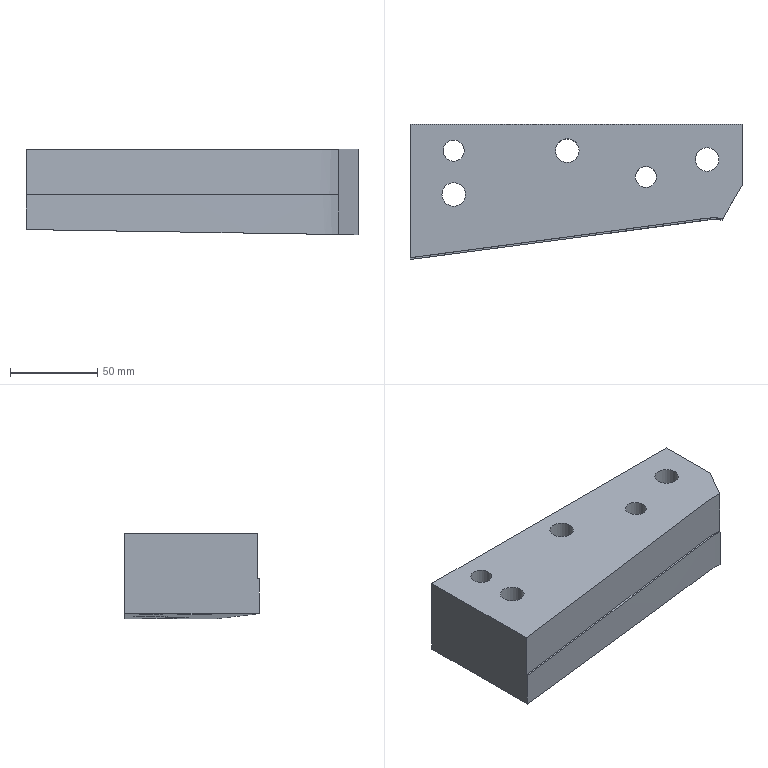Part | NX | features solid 2 | 1 solid | 24 faces | box 190 x 77.202 x 49 mm | volume 533437 mm3 | plane 12 | cylinder 10 | spline 2 | commonest cylinder face diameters 13.5 x3 19.5 x3 12 x2 13 x2
STEP:
#1=CARTESIAN_POINT('',(309.118,134.287,40.));
#2=VERTEX_POINT('',#1);
#3=CARTESIAN_POINT('',(130.,111.807,40.));
#4=VERTEX_POINT('',#3);
#5=CARTESIAN_POINT('',(309.118,134.287,40.));
#6=CARTESIAN_POINT('',(307.251,134.588,40.));
#7=CARTESIAN_POINT('',(303.399,134.795,40.));
#8=CARTESIAN_POINT('',(297.809,134.152,40.));
#9=CARTESIAN_POINT('',(292.221,133.323,40.));
#10=CARTESIAN_POINT('',(284.77,132.284,40.));
#11=CARTESIAN_POINT('',(275.453,130.997,40.));
#12=CARTESIAN_POINT('',(264.266,129.504,40.));
#13=CARTESIAN_POINT('',(253.078,128.021,40.));
#14=CARTESIAN_POINT('',(238.16,126.052,40.));
#15=CARTESIAN_POINT('',(219.511,123.602,40.));
#16=CARTESIAN_POINT('',(197.131,120.668,40.));
#17=CARTESIAN_POINT('',(167.294,116.739,40.));
#18=CARTESIAN_POINT('',(144.918,113.773,40.));
#19=CARTESIAN_POINT('',(130.,111.807,40.));
#20=B_SPLINE_CURVE_WITH_KNOTS('',3,(#5,#6,#7,#8,#9,#10,#11,#12,#13,#14,#15,#16,#17,#18,#19),.UNSPECIFIED.,.F.,.F.,(4,1,1,1,1,1,1,1,1,1,1,1,4),(0.01153,0.01714,0.02276,0.02838,0.034,0.04523,0.05646,0.0677,0.07893,0.1014,0.1239,0.1463,0.1913),.UNSPECIFIED.);
#21=EDGE_CURVE('',#2,#4,#20,.T.);
#22=ORIENTED_EDGE('',*,*,#21,.F.);
#23=CARTESIAN_POINT('',(320.,153.135,40.));
#24=VERTEX_POINT('',#23);
#25=CARTESIAN_POINT('',(85.016,-253.87,40.));
#26=DIRECTION('',(0.5,0.866,0.));
#27=VECTOR('',#26,1000.);
#28=LINE('',#25,#27);
#29=EDGE_CURVE('',#2,#24,#28,.T.);
#30=ORIENTED_EDGE('',*,*,#29,.T.);
#31=CARTESIAN_POINT('',(320.,188.,40.));
#32=VERTEX_POINT('',#31);
#33=CARTESIAN_POINT('',(320.,35.09,40.));
#34=DIRECTION('',(0.,1.,0.));
#35=VECTOR('',#34,1000.);
#36=LINE('',#33,#35);
#37=EDGE_CURVE('',#24,#32,#36,.T.);
#38=ORIENTED_EDGE('',*,*,#37,.T.);
#39=CARTESIAN_POINT('',(130.,188.,40.));
#40=VERTEX_POINT('',#39);
#41=CARTESIAN_POINT('',(-415.478,188.,40.));
#42=DIRECTION('',(1.,0.,0.));
#43=VECTOR('',#42,1000.);
#44=LINE('',#41,#43);
#45=EDGE_CURVE('',#40,#32,#44,.T.);
#46=ORIENTED_EDGE('',*,*,#45,.F.);
#47=CARTESIAN_POINT('',(130.,35.09,40.));
#48=DIRECTION('',(0.,1.,0.));
#49=VECTOR('',#48,1000.);
#50=LINE('',#47,#49);
#51=EDGE_CURVE('',#4,#40,#50,.T.);
#52=ORIENTED_EDGE('',*,*,#51,.F.);
#53=EDGE_LOOP('',(#22,#30,#38,#46,#52));
#54=FACE_BOUND('',#53,.T.);
#55=CARTESIAN_POINT('',(271.,158.,40.));
#56=VERTEX_POINT('',#55);
#57=CARTESIAN_POINT('',(265.,158.,40.));
#58=DIRECTION('',(0.,0.,1.));
#59=DIRECTION('',(1.,0.,0.));
#60=AXIS2_PLACEMENT_3D('',#57,#58,#59);
#61=CIRCLE('',#60,6.);
#62=EDGE_CURVE('',#56,#56,#61,.T.);
#63=ORIENTED_EDGE('',*,*,#62,.F.);
#64=EDGE_LOOP('',(#63));
#65=FACE_BOUND('',#64,.T.);
#66=CARTESIAN_POINT('',(161.,173.,40.));
#67=VERTEX_POINT('',#66);
#68=CARTESIAN_POINT('',(155.,173.,40.));
#69=DIRECTION('',(0.,0.,1.));
#70=DIRECTION('',(1.,0.,0.));
#71=AXIS2_PLACEMENT_3D('',#68,#69,#70);
#72=CIRCLE('',#71,6.);
#73=EDGE_CURVE('',#67,#67,#72,.T.);
#74=ORIENTED_EDGE('',*,*,#73,.F.);
#75=EDGE_LOOP('',(#74));
#76=FACE_BOUND('',#75,.T.);
#77=CARTESIAN_POINT('',(226.75,173.,40.));
#78=VERTEX_POINT('',#77);
#79=CARTESIAN_POINT('',(220.,173.,40.));
#80=DIRECTION('',(0.,0.,1.));
#81=DIRECTION('',(1.,0.,0.));
#82=AXIS2_PLACEMENT_3D('',#79,#80,#81);
#83=CIRCLE('',#82,6.75);
#84=EDGE_CURVE('',#78,#78,#83,.T.);
#85=ORIENTED_EDGE('',*,*,#84,.F.);
#86=EDGE_LOOP('',(#85));
#87=FACE_BOUND('',#86,.T.);
#88=CARTESIAN_POINT('',(161.75,148.,40.));
#89=VERTEX_POINT('',#88);
#90=CARTESIAN_POINT('',(155.,148.,40.));
#91=DIRECTION('',(0.,0.,1.));
#92=DIRECTION('',(1.,0.,0.));
#93=AXIS2_PLACEMENT_3D('',#90,#91,#92);
#94=CIRCLE('',#93,6.75);
#95=EDGE_CURVE('',#89,#89,#94,.T.);
#96=ORIENTED_EDGE('',*,*,#95,.F.);
#97=EDGE_LOOP('',(#96));
#98=FACE_BOUND('',#97,.T.);
#99=CARTESIAN_POINT('',(306.75,168.,40.));
#100=VERTEX_POINT('',#99);
#101=CARTESIAN_POINT('',(300.,168.,40.));
#102=DIRECTION('',(0.,0.,1.));
#103=DIRECTION('',(1.,0.,0.));
#104=AXIS2_PLACEMENT_3D('',#101,#102,#103);
#105=CIRCLE('',#104,6.75);
#106=EDGE_CURVE('',#100,#100,#105,.T.);
#107=ORIENTED_EDGE('',*,*,#106,.F.);
#108=EDGE_LOOP('',(#107));
#109=FACE_BOUND('',#108,.T.);
#110=CARTESIAN_POINT('',(-415.478,35.09,40.));
#111=DIRECTION('',(0.,0.,1.));
#112=DIRECTION('',(1.,0.,0.));
#113=AXIS2_PLACEMENT_3D('',#110,#111,#112);
#114=PLANE('',#113);
#115=ADVANCED_FACE('',(#54,#65,#76,#87,#98,#109),#114,.T.);
#116=CARTESIAN_POINT('',(320.,153.135,-9.));
#117=VERTEX_POINT('',#116);
#118=CARTESIAN_POINT('',(320.,153.135,23.));
#119=DIRECTION('',(0.,0.,1.));
#120=VECTOR('',#119,1000.);
#121=LINE('',#118,#120);
#122=EDGE_CURVE('',#117,#24,#121,.T.);
#123=ORIENTED_EDGE('',*,*,#122,.F.);
#124=CARTESIAN_POINT('',(320.,188.,-9.));
#125=VERTEX_POINT('',#124);
#126=CARTESIAN_POINT('',(320.,-222.,-9.));
#127=DIRECTION('',(0.,-1.,0.));
#128=VECTOR('',#127,1000.);
#129=LINE('',#126,#128);
#130=EDGE_CURVE('',#125,#117,#129,.T.);
#131=ORIENTED_EDGE('',*,*,#130,.F.);
#132=CARTESIAN_POINT('',(320.,188.,-206.));
#133=DIRECTION('',(0.,0.,1.));
#134=VECTOR('',#133,1000.);
#135=LINE('',#132,#134);
#136=EDGE_CURVE('',#125,#32,#135,.T.);
#137=ORIENTED_EDGE('',*,*,#136,.T.);
#138=ORIENTED_EDGE('',*,*,#37,.F.);
#139=EDGE_LOOP('',(#123,#131,#137,#138));
#140=FACE_BOUND('',#139,.T.);
#141=CARTESIAN_POINT('',(320.,105.,2.));
#142=DIRECTION('',(1.,0.,0.));
#143=DIRECTION('',(0.,0.,-1.));
#144=AXIS2_PLACEMENT_3D('',#141,#142,#143);
#145=PLANE('',#144);
#146=ADVANCED_FACE('',(#140),#145,.T.);
#147=CARTESIAN_POINT('',(308.582,133.358,14.));
#148=VERTEX_POINT('',#147);
#149=CARTESIAN_POINT('',(309.118,134.287,14.));
#150=VERTEX_POINT('',#149);
#151=CARTESIAN_POINT('',(326.746,164.819,14.));
#152=DIRECTION('',(0.5,0.866,0.));
#153=VECTOR('',#152,1000.);
#154=LINE('',#151,#153);
#155=EDGE_CURVE('',#148,#150,#154,.T.);
#156=ORIENTED_EDGE('',*,*,#155,.F.);
#157=CARTESIAN_POINT('',(308.582,133.358,-8.82));
#158=VERTEX_POINT('',#157);
#159=CARTESIAN_POINT('',(308.582,133.358,2.57));
#160=DIRECTION('',(0.,0.,-1.));
#161=VECTOR('',#160,1000.);
#162=LINE('',#159,#161);
#163=EDGE_CURVE('',#158,#148,#162,.F.);
#164=ORIENTED_EDGE('',*,*,#163,.F.);
#165=CARTESIAN_POINT('',(-40.023,-470.443,-3.315));
#166=DIRECTION('',(-0.5,-0.866,0.007894));
#167=VECTOR('',#166,1000.);
#168=LINE('',#165,#167);
#169=EDGE_CURVE('',#117,#158,#168,.T.);
#170=ORIENTED_EDGE('',*,*,#169,.F.);
#171=ORIENTED_EDGE('',*,*,#122,.T.);
#172=ORIENTED_EDGE('',*,*,#29,.F.);
#173=CARTESIAN_POINT('',(309.118,134.287,57.));
#174=DIRECTION('',(0.,0.,1.));
#175=VECTOR('',#174,1000.);
#176=LINE('',#173,#175);
#177=EDGE_CURVE('',#150,#2,#176,.T.);
#178=ORIENTED_EDGE('',*,*,#177,.F.);
#179=EDGE_LOOP('',(#156,#164,#170,#171,#172,#178));
#180=FACE_BOUND('',#179,.T.);
#181=CARTESIAN_POINT('',(326.746,164.819,23.));
#182=DIRECTION('',(0.866,-0.5,0.));
#183=DIRECTION('',(0.5,0.866,0.));
#184=AXIS2_PLACEMENT_3D('',#181,#182,#183);
#185=PLANE('',#184);
#186=ADVANCED_FACE('',(#180),#185,.T.);
#187=ORIENTED_EDGE('',*,*,#136,.F.);
#188=CARTESIAN_POINT('',(130.,188.,-6.));
#189=VERTEX_POINT('',#188);
#190=CARTESIAN_POINT('',(-470.225,188.,3.477));
#191=DIRECTION('',(0.9999,0.,-0.01579));
#192=VECTOR('',#191,1000.);
#193=LINE('',#190,#192);
#194=EDGE_CURVE('',#189,#125,#193,.T.);
#195=ORIENTED_EDGE('',*,*,#194,.F.);
#196=CARTESIAN_POINT('',(130.,188.,-206.));
#197=DIRECTION('',(0.,0.,1.));
#198=VECTOR('',#197,1000.);
#199=LINE('',#196,#198);
#200=EDGE_CURVE('',#189,#40,#199,.T.);
#201=ORIENTED_EDGE('',*,*,#200,.T.);
#202=ORIENTED_EDGE('',*,*,#45,.T.);
#203=EDGE_LOOP('',(#187,#195,#201,#202));
#204=FACE_BOUND('',#203,.T.);
#205=CARTESIAN_POINT('',(-470.374,188.,-206.));
#206=DIRECTION('',(0.,-1.,0.));
#207=DIRECTION('',(1.,0.,0.));
#208=AXIS2_PLACEMENT_3D('',#205,#206,#207);
#209=PLANE('',#208);
#210=ADVANCED_FACE('',(#204),#209,.F.);
#211=CARTESIAN_POINT('',(130.,110.798,14.));
#212=VERTEX_POINT('',#211);
#213=CARTESIAN_POINT('',(-190.231,-121.49,14.));
#214=CARTESIAN_POINT('',(-188.654,-121.152,14.));
#215=CARTESIAN_POINT('',(-185.47,-120.627,14.));
#216=CARTESIAN_POINT('',(-180.656,-120.141,14.));
#217=CARTESIAN_POINT('',(-175.882,-119.326,14.));
#218=CARTESIAN_POINT('',(-169.679,-117.528,14.));
#219=CARTESIAN_POINT('',(-162.185,-114.539,14.));
#220=CARTESIAN_POINT('',(-153.086,-111.254,14.));
#221=CARTESIAN_POINT('',(-144.031,-107.845,14.));
#222=CARTESIAN_POINT('',(-136.465,-105.061,14.));
#223=CARTESIAN_POINT('',(-130.418,-102.814,14.));
#224=CARTESIAN_POINT('',(-125.812,-101.329,14.));
#225=CARTESIAN_POINT('',(-121.306,-99.566,14.));
#226=CARTESIAN_POINT('',(-116.876,-97.626,14.));
#227=CARTESIAN_POINT('',(-112.335,-95.923,14.));
#228=CARTESIAN_POINT('',(-107.564,-95.05,14.));
#229=CARTESIAN_POINT('',(-102.756,-94.525,14.));
#230=CARTESIAN_POINT('',(-96.349,-93.771,14.));
#231=CARTESIAN_POINT('',(-89.902,-93.468,14.));
#232=CARTESIAN_POINT('',(-83.452,-93.448,14.));
#233=CARTESIAN_POINT('',(-77.002,-93.469,14.));
#234=CARTESIAN_POINT('',(-68.939,-93.411,14.));
#235=CARTESIAN_POINT('',(-56.04,-93.3,14.));
#236=CARTESIAN_POINT('',(-33.465,-93.184,14.));
#237=CARTESIAN_POINT('',(-7.666,-93.074,14.));
#238=CARTESIAN_POINT('',(14.907,-92.653,14.));
#239=CARTESIAN_POINT('',(27.794,-92.068,14.));
#240=CARTESIAN_POINT('',(40.668,-91.245,14.));
#241=CARTESIAN_POINT('',(51.917,-90.291,14.));
#242=CARTESIAN_POINT('',(61.528,-89.174,14.));
#243=CARTESIAN_POINT('',(67.939,-88.466,14.));
#244=CARTESIAN_POINT('',(79.125,-86.95,14.));
#245=CARTESIAN_POINT('',(95.161,-85.253,14.));
#246=CARTESIAN_POINT('',(114.404,-83.21,14.));
#247=CARTESIAN_POINT('',(133.568,-80.524,14.));
#248=CARTESIAN_POINT('',(152.734,-77.861,14.));
#249=CARTESIAN_POINT('',(171.916,-75.326,14.));
#250=CARTESIAN_POINT('',(191.055,-72.413,14.));
#251=CARTESIAN_POINT('',(207.17,-71.468,14.));
#252=CARTESIAN_POINT('',(219.951,-69.697,14.));
#253=CARTESIAN_POINT('',(232.724,-67.899,14.));
#254=CARTESIAN_POINT('',(248.708,-65.766,14.));
#255=CARTESIAN_POINT('',(267.87,-63.074,14.));
#256=CARTESIAN_POINT('',(287.038,-60.44,14.));
#257=CARTESIAN_POINT('',(301.448,-58.682,14.));
#258=CARTESIAN_POINT('',(310.976,-56.987,14.));
#259=CARTESIAN_POINT('',(314.916,-56.135,14.));
#260=CARTESIAN_POINT('',(318.052,-55.382,14.));
#261=CARTESIAN_POINT('',(320.39,-54.76,14.));
#262=CARTESIAN_POINT('',(322.686,-53.981,14.));
#263=CARTESIAN_POINT('',(325.595,-52.578,14.));
#264=CARTESIAN_POINT('',(328.769,-50.098,14.));
#265=CARTESIAN_POINT('',(332.247,-46.69,14.));
#266=CARTESIAN_POINT('',(335.795,-43.406,14.));
#267=CARTESIAN_POINT('',(343.661,-37.758,14.));
#268=CARTESIAN_POINT('',(355.164,-28.914,14.));
#269=CARTESIAN_POINT('',(370.422,-17.018,14.));
#270=CARTESIAN_POINT('',(383.264,-7.249,14.));
#271=CARTESIAN_POINT('',(392.416,-0.6713,14.));
#272=CARTESIAN_POINT('',(396.953,2.733,14.));
#273=CARTESIAN_POINT('',(398.886,5.372,14.));
#274=CARTESIAN_POINT('',(399.725,7.654,14.));
#275=CARTESIAN_POINT('',(399.76,10.078,14.));
#276=CARTESIAN_POINT('',(399.483,13.317,14.));
#277=CARTESIAN_POINT('',(399.712,17.34,14.));
#278=CARTESIAN_POINT('',(399.612,22.179,14.));
#279=CARTESIAN_POINT('',(399.633,31.854,14.));
#280=CARTESIAN_POINT('',(399.593,46.366,14.));
#281=CARTESIAN_POINT('',(399.637,62.491,14.));
#282=CARTESIAN_POINT('',(399.588,73.779,14.));
#283=CARTESIAN_POINT('',(399.652,79.422,14.));
#284=CARTESIAN_POINT('',(399.59,82.647,14.));
#285=CARTESIAN_POINT('',(399.564,85.065,14.));
#286=CARTESIAN_POINT('',(399.725,87.486,14.));
#287=CARTESIAN_POINT('',(399.756,89.902,14.));
#288=CARTESIAN_POINT('',(399.247,92.301,14.));
#289=CARTESIAN_POINT('',(397.362,95.008,14.));
#290=CARTESIAN_POINT('',(393.635,96.774,14.));
#291=CARTESIAN_POINT('',(389.279,98.826,14.));
#292=CARTESIAN_POINT('',(384.732,100.498,14.));
#293=CARTESIAN_POINT('',(378.765,102.95,14.));
#294=CARTESIAN_POINT('',(362.589,110.229,14.));
#295=CARTESIAN_POINT('',(344.928,118.135,14.));
#296=CARTESIAN_POINT('',(327.281,126.072,14.));
#297=CARTESIAN_POINT('',(319.932,129.381,14.));
#298=CARTESIAN_POINT('',(314.075,132.102,14.));
#299=CARTESIAN_POINT('',(309.387,133.376,14.));
#300=CARTESIAN_POINT('',(304.547,133.785,14.));
#301=CARTESIAN_POINT('',(299.716,133.401,14.));
#302=CARTESIAN_POINT('',(294.929,132.704,14.));
#303=CARTESIAN_POINT('',(288.543,131.8,14.));
#304=CARTESIAN_POINT('',(277.364,130.241,14.));
#305=CARTESIAN_POINT('',(242.2,125.552,14.));
#306=CARTESIAN_POINT('',(184.637,118.048,14.));
#307=CARTESIAN_POINT('',(120.701,109.541,14.));
#308=CARTESIAN_POINT('',(69.531,102.902,14.));
#309=CARTESIAN_POINT('',(40.777,98.94,14.));
#310=CARTESIAN_POINT('',(21.566,96.615,14.));
#311=CARTESIAN_POINT('',(8.743,95.212,14.));
#312=CARTESIAN_POINT('',(-7.301,93.575,14.));
#313=CARTESIAN_POINT('',(-26.625,92.505,14.));
#314=CARTESIAN_POINT('',(-45.971,92.017,14.));
#315=CARTESIAN_POINT('',(-62.09,91.675,14.));
#316=CARTESIAN_POINT('',(-74.987,91.256,14.));
#317=CARTESIAN_POINT('',(-84.664,91.165,14.));
#318=CARTESIAN_POINT('',(-94.319,91.781,14.));
#319=CARTESIAN_POINT('',(-103.929,92.966,14.));
#320=CARTESIAN_POINT('',(-113.495,94.403,14.));
#321=CARTESIAN_POINT('',(-119.856,95.492,14.));
#322=CARTESIAN_POINT('',(-122.997,96.222,14.));
#323=B_SPLINE_CURVE_WITH_KNOTS('',3,(#213,#214,#215,#216,#217,#218,#219,#220,#221,#222,#223,#224,#225,#226,#227,#228,#229,#230,#231,#232,#233,#234,#235,#236,#237,#238,#239,#240,#241,#242,#243,#244,#245,#246,#247,#248,#249,#250,#251,#252,#253,#254,#255,#256,#257,#258,#259,#260,#261,#262,#263,#264,#265,#266,#267,#268,#269,#270,#271,#272,#273,#274,#275,#276,#277,#278,#279,#280,#281,#282,#283,#284,#285,#286,#287,#288,#289,#290,#291,#292,#293,#294,#295,#296,#297,#298,#299,#300,#301,#302,#303,#304,#305,#306,#307,#308,#309,#310,#311,#312,#313,#314,#315,#316,#317,#318,#319,#320,#321,#322),.UNSPECIFIED.,.F.,.F.,(4,1,1,1,1,1,1,1,1,1,1,1,1,1,1,1,1,1,1,1,1,1,1,1,1,1,1,1,1,1,1,1,1,1,1,1,1,1,1,1,1,1,1,1,1,1,1,1,1,1,1,1,1,1,1,1,1,1,1,1,1,1,1,1,1,1,1,1,1,1,1,1,1,1,1,1,1,1,1,1,1,1,1,1,1,1,1,1,1,1,1,1,1,1,1,1,1,1,1,1,1,1,1,1,1,1,1,4),(0.4704,0.4724,0.4745,0.4766,0.4786,0.4828,0.4869,0.491,0.4952,0.4972,0.4993,0.5014,0.5035,0.5055,0.5076,0.5097,0.5117,0.5159,0.5179,0.52,0.5241,0.5283,0.5366,0.5531,0.5614,0.5655,0.5697,0.5779,0.58,0.5821,0.5862,0.5945,0.6028,0.611,0.6193,0.6276,0.6359,0.6441,0.6483,0.6524,0.6607,0.669,0.6772,0.6855,0.6876,0.6897,0.6907,0.6917,0.6928,0.6938,0.6959,0.6979,0.7,0.7021,0.7103,0.7186,0.7269,0.731,0.7331,0.7341,0.7352,0.7362,0.7372,0.7393,0.7414,0.7435,0.7517,0.76,0.7641,0.7662,0.7672,0.7683,0.7693,0.7703,0.7714,0.7724,0.7745,0.7766,0.7786,0.7807,0.7848,0.8014,0.8055,0.8097,0.8117,0.8138,0.8159,0.8179,0.82,0.8221,0.8262,0.8345,0.8676,0.9007,0.9172,0.9338,0.9379,0.9421,0.9503,0.9586,0.9669,0.9752,0.9793,0.9834,0.9876,0.9917,0.9959,1.),.UNSPECIFIED.);
#324=EDGE_CURVE('',#212,#148,#323,.F.);
#325=ORIENTED_EDGE('',*,*,#324,.F.);
#326=CARTESIAN_POINT('',(130.,110.798,-6.));
#327=VERTEX_POINT('',#326);
#328=CARTESIAN_POINT('',(130.,110.798,4.));
#329=DIRECTION('',(0.,0.,-1.));
#330=VECTOR('',#329,1000.);
#331=LINE('',#328,#330);
#332=EDGE_CURVE('',#327,#212,#331,.F.);
#333=ORIENTED_EDGE('',*,*,#332,.F.);
#334=CARTESIAN_POINT('',(130.,110.798,-6.));
#335=CARTESIAN_POINT('',(144.872,112.758,-6.235));
#336=CARTESIAN_POINT('',(167.177,115.715,-6.587));
#337=CARTESIAN_POINT('',(196.921,119.631,-7.057));
#338=CARTESIAN_POINT('',(219.23,122.557,-7.409));
#339=CARTESIAN_POINT('',(237.821,124.999,-7.702));
#340=CARTESIAN_POINT('',(252.692,126.962,-7.937));
#341=CARTESIAN_POINT('',(263.845,128.438,-8.113));
#342=CARTESIAN_POINT('',(274.996,129.934,-8.289));
#343=CARTESIAN_POINT('',(286.146,131.436,-8.465));
#344=CARTESIAN_POINT('',(297.272,133.122,-8.641));
#345=CARTESIAN_POINT('',(304.731,133.922,-8.759));
#346=CARTESIAN_POINT('',(308.582,133.358,-8.82));
#347=B_SPLINE_CURVE_WITH_KNOTS('',3,(#334,#335,#336,#337,#338,#339,#340,#341,#342,#343,#344,#345,#346),.UNSPECIFIED.,.F.,.F.,(4,1,1,1,1,1,1,1,1,1,4),(0.,0.04501,0.06751,0.09001,0.1125,0.1238,0.135,0.1463,0.1575,0.1688,0.18),.UNSPECIFIED.);
#348=EDGE_CURVE('',#327,#158,#347,.T.);
#349=ORIENTED_EDGE('',*,*,#348,.T.);
#350=ORIENTED_EDGE('',*,*,#163,.T.);
#351=EDGE_LOOP('',(#325,#333,#349,#350));
#352=FACE_BOUND('',#351,.T.);
#353=CARTESIAN_POINT('',(308.582,133.358,14.));
#354=CARTESIAN_POINT('',(308.582,133.358,-8.957));
#355=CARTESIAN_POINT('',(306.726,133.63,14.));
#356=CARTESIAN_POINT('',(306.726,133.63,-8.957));
#357=CARTESIAN_POINT('',(302.961,133.768,14.));
#358=CARTESIAN_POINT('',(302.961,133.768,-8.957));
#359=CARTESIAN_POINT('',(297.366,133.074,14.));
#360=CARTESIAN_POINT('',(297.366,133.074,-8.957));
#361=CARTESIAN_POINT('',(291.8,132.254,14.));
#362=CARTESIAN_POINT('',(291.8,132.254,-8.957));
#363=CARTESIAN_POINT('',(284.367,131.218,14.));
#364=CARTESIAN_POINT('',(284.367,131.218,-8.957));
#365=CARTESIAN_POINT('',(275.075,129.937,14.));
#366=CARTESIAN_POINT('',(275.075,129.937,-8.957));
#367=CARTESIAN_POINT('',(263.917,128.449,14.));
#368=CARTESIAN_POINT('',(263.917,128.449,-8.957));
#369=CARTESIAN_POINT('',(252.759,126.97,14.));
#370=CARTESIAN_POINT('',(252.759,126.97,-8.957));
#371=CARTESIAN_POINT('',(237.879,125.006,14.));
#372=CARTESIAN_POINT('',(237.879,125.006,-8.957));
#373=CARTESIAN_POINT('',(219.279,122.563,14.));
#374=CARTESIAN_POINT('',(219.279,122.563,-8.957));
#375=CARTESIAN_POINT('',(196.957,119.636,14.));
#376=CARTESIAN_POINT('',(196.957,119.636,-8.957));
#377=CARTESIAN_POINT('',(167.197,115.718,14.));
#378=CARTESIAN_POINT('',(167.197,115.718,-8.957));
#379=CARTESIAN_POINT('',(144.88,112.759,14.));
#380=CARTESIAN_POINT('',(144.88,112.759,-8.957));
#381=CARTESIAN_POINT('',(130.,110.798,14.));
#382=CARTESIAN_POINT('',(130.,110.798,-8.957));
#383=B_SPLINE_SURFACE_WITH_KNOTS('',3,1,((#353,#354),(#355,#356),(#357,#358),(#359,#360),(#361,#362),(#363,#364),(#365,#366),(#367,#368),(#369,#370),(#371,#372),(#373,#374),(#375,#376),(#377,#378),(#379,#380),(#381,#382)),.SURF_OF_LINEAR_EXTRUSION.,.F.,.F.,.F.,(4,1,1,1,1,1,1,1,1,1,1,1,4),(2,2),(0.8141,0.8165,0.8189,0.8214,0.8238,0.8286,0.8334,0.8382,0.843,0.8526,0.8623,0.8719,0.8912),(0.,1.),.UNSPECIFIED.);
#384=ADVANCED_FACE('',(#352),#383,.T.);
#385=ORIENTED_EDGE('',*,*,#332,.T.);
#386=CARTESIAN_POINT('',(130.,111.807,14.));
#387=VERTEX_POINT('',#386);
#388=CARTESIAN_POINT('',(130.,154.403,14.));
#389=DIRECTION('',(0.,1.,0.));
#390=VECTOR('',#389,1000.);
#391=LINE('',#388,#390);
#392=EDGE_CURVE('',#212,#387,#391,.T.);
#393=ORIENTED_EDGE('',*,*,#392,.T.);
#394=CARTESIAN_POINT('',(130.,111.807,57.));
#395=DIRECTION('',(0.,0.,1.));
#396=VECTOR('',#395,1000.);
#397=LINE('',#394,#396);
#398=EDGE_CURVE('',#387,#4,#397,.T.);
#399=ORIENTED_EDGE('',*,*,#398,.T.);
#400=ORIENTED_EDGE('',*,*,#51,.T.);
#401=ORIENTED_EDGE('',*,*,#200,.F.);
#402=CARTESIAN_POINT('',(130.,-222.,-6.));
#403=DIRECTION('',(0.,-1.,0.));
#404=VECTOR('',#403,1000.);
#405=LINE('',#402,#404);
#406=EDGE_CURVE('',#189,#327,#405,.T.);
#407=ORIENTED_EDGE('',*,*,#406,.T.);
#408=EDGE_LOOP('',(#385,#393,#399,#400,#401,#407));
#409=FACE_BOUND('',#408,.T.);
#410=CARTESIAN_POINT('',(130.,154.403,21.5));
#411=DIRECTION('',(1.,0.,0.));
#412=DIRECTION('',(0.,0.,-1.));
#413=AXIS2_PLACEMENT_3D('',#410,#411,#412);
#414=PLANE('',#413);
#415=ADVANCED_FACE('',(#409),#414,.F.);
#416=ORIENTED_EDGE('',*,*,#106,.T.);
#417=EDGE_LOOP('',(#416));
#418=FACE_BOUND('',#417,.T.);
#419=CARTESIAN_POINT('',(306.75,168.,9.));
#420=VERTEX_POINT('',#419);
#421=CARTESIAN_POINT('',(300.,168.,9.));
#422=DIRECTION('',(0.,0.,1.));
#423=DIRECTION('',(1.,0.,0.));
#424=AXIS2_PLACEMENT_3D('',#421,#422,#423);
#425=CIRCLE('',#424,6.75);
#426=EDGE_CURVE('',#420,#420,#425,.T.);
#427=ORIENTED_EDGE('',*,*,#426,.F.);
#428=EDGE_LOOP('',(#427));
#429=FACE_BOUND('',#428,.T.);
#430=CARTESIAN_POINT('',(300.,168.,94.));
#431=DIRECTION('',(0.,0.,1.));
#432=DIRECTION('',(1.,0.,0.));
#433=AXIS2_PLACEMENT_3D('',#430,#431,#432);
#434=CYLINDRICAL_SURFACE('',#433,6.75);
#435=ADVANCED_FACE('',(#418,#429),#434,.F.);
#436=ORIENTED_EDGE('',*,*,#426,.T.);
#437=EDGE_LOOP('',(#436));
#438=FACE_BOUND('',#437,.T.);
#439=CARTESIAN_POINT('',(309.75,168.,9.));
#440=VERTEX_POINT('',#439);
#441=CARTESIAN_POINT('',(300.,168.,9.));
#442=DIRECTION('',(0.,0.,1.));
#443=DIRECTION('',(1.,0.,0.));
#444=AXIS2_PLACEMENT_3D('',#441,#442,#443);
#445=CIRCLE('',#444,9.75);
#446=EDGE_CURVE('',#440,#440,#445,.T.);
#447=ORIENTED_EDGE('',*,*,#446,.F.);
#448=EDGE_LOOP('',(#447));
#449=FACE_BOUND('',#448,.T.);
#450=CARTESIAN_POINT('',(300.,168.,9.));
#451=DIRECTION('',(0.,0.,1.));
#452=DIRECTION('',(1.,0.,0.));
#453=AXIS2_PLACEMENT_3D('',#450,#451,#452);
#454=PLANE('',#453);
#455=ADVANCED_FACE('',(#438,#449),#454,.F.);
#456=ORIENTED_EDGE('',*,*,#446,.T.);
#457=EDGE_LOOP('',(#456));
#458=FACE_BOUND('',#457,.T.);
#459=CARTESIAN_POINT('',(309.75,168.,-8.838));
#460=VERTEX_POINT('',#459);
#461=CARTESIAN_POINT('',(300.,168.,-8.684));
#462=DIRECTION('',(0.01579,0.,0.9999));
#463=DIRECTION('',(0.9999,0.,-0.01579));
#464=AXIS2_PLACEMENT_3D('',#461,#462,#463);
#465=ELLIPSE('',#464,9.751,9.75);
#466=EDGE_CURVE('',#460,#460,#465,.T.);
#467=ORIENTED_EDGE('',*,*,#466,.F.);
#468=EDGE_LOOP('',(#467));
#469=FACE_BOUND('',#468,.T.);
#470=CARTESIAN_POINT('',(300.,168.,-6.));
#471=DIRECTION('',(0.,0.,1.));
#472=DIRECTION('',(1.,0.,0.));
#473=AXIS2_PLACEMENT_3D('',#470,#471,#472);
#474=CYLINDRICAL_SURFACE('',#473,9.75);
#475=ADVANCED_FACE('',(#458,#469),#474,.F.);
#476=ORIENTED_EDGE('',*,*,#95,.T.);
#477=EDGE_LOOP('',(#476));
#478=FACE_BOUND('',#477,.T.);
#479=CARTESIAN_POINT('',(161.75,148.,9.));
#480=VERTEX_POINT('',#479);
#481=CARTESIAN_POINT('',(155.,148.,9.));
#482=DIRECTION('',(0.,0.,1.));
#483=DIRECTION('',(1.,0.,0.));
#484=AXIS2_PLACEMENT_3D('',#481,#482,#483);
#485=CIRCLE('',#484,6.75);
#486=EDGE_CURVE('',#480,#480,#485,.T.);
#487=ORIENTED_EDGE('',*,*,#486,.F.);
#488=EDGE_LOOP('',(#487));
#489=FACE_BOUND('',#488,.T.);
#490=CARTESIAN_POINT('',(155.,148.,94.));
#491=DIRECTION('',(0.,0.,1.));
#492=DIRECTION('',(1.,0.,0.));
#493=AXIS2_PLACEMENT_3D('',#490,#491,#492);
#494=CYLINDRICAL_SURFACE('',#493,6.75);
#495=ADVANCED_FACE('',(#478,#489),#494,.F.);
#496=ORIENTED_EDGE('',*,*,#486,.T.);
#497=EDGE_LOOP('',(#496));
#498=FACE_BOUND('',#497,.T.);
#499=CARTESIAN_POINT('',(164.75,148.,9.));
#500=VERTEX_POINT('',#499);
#501=CARTESIAN_POINT('',(155.,148.,9.));
#502=DIRECTION('',(0.,0.,1.));
#503=DIRECTION('',(1.,0.,0.));
#504=AXIS2_PLACEMENT_3D('',#501,#502,#503);
#505=CIRCLE('',#504,9.75);
#506=EDGE_CURVE('',#500,#500,#505,.T.);
#507=ORIENTED_EDGE('',*,*,#506,.F.);
#508=EDGE_LOOP('',(#507));
#509=FACE_BOUND('',#508,.T.);
#510=CARTESIAN_POINT('',(155.,148.,9.));
#511=DIRECTION('',(0.,0.,1.));
#512=DIRECTION('',(1.,0.,0.));
#513=AXIS2_PLACEMENT_3D('',#510,#511,#512);
#514=PLANE('',#513);
#515=ADVANCED_FACE('',(#498,#509),#514,.F.);
#516=ORIENTED_EDGE('',*,*,#506,.T.);
#517=EDGE_LOOP('',(#516));
#518=FACE_BOUND('',#517,.T.);
#519=CARTESIAN_POINT('',(164.75,148.,-6.549));
#520=VERTEX_POINT('',#519);
#521=CARTESIAN_POINT('',(155.,148.,-6.395));
#522=DIRECTION('',(0.01579,0.,0.9999));
#523=DIRECTION('',(0.9999,0.,-0.01579));
#524=AXIS2_PLACEMENT_3D('',#521,#522,#523);
#525=ELLIPSE('',#524,9.751,9.75);
#526=EDGE_CURVE('',#520,#520,#525,.T.);
#527=ORIENTED_EDGE('',*,*,#526,.F.);
#528=EDGE_LOOP('',(#527));
#529=FACE_BOUND('',#528,.T.);
#530=CARTESIAN_POINT('',(155.,148.,-6.));
#531=DIRECTION('',(0.,0.,1.));
#532=DIRECTION('',(1.,0.,0.));
#533=AXIS2_PLACEMENT_3D('',#530,#531,#532);
#534=CYLINDRICAL_SURFACE('',#533,9.75);
#535=ADVANCED_FACE('',(#518,#529),#534,.F.);
#536=ORIENTED_EDGE('',*,*,#84,.T.);
#537=EDGE_LOOP('',(#536));
#538=FACE_BOUND('',#537,.T.);
#539=CARTESIAN_POINT('',(226.75,173.,9.));
#540=VERTEX_POINT('',#539);
#541=CARTESIAN_POINT('',(220.,173.,9.));
#542=DIRECTION('',(0.,0.,1.));
#543=DIRECTION('',(1.,0.,0.));
#544=AXIS2_PLACEMENT_3D('',#541,#542,#543);
#545=CIRCLE('',#544,6.75);
#546=EDGE_CURVE('',#540,#540,#545,.T.);
#547=ORIENTED_EDGE('',*,*,#546,.F.);
#548=EDGE_LOOP('',(#547));
#549=FACE_BOUND('',#548,.T.);
#550=CARTESIAN_POINT('',(220.,173.,94.));
#551=DIRECTION('',(0.,0.,1.));
#552=DIRECTION('',(1.,0.,0.));
#553=AXIS2_PLACEMENT_3D('',#550,#551,#552);
#554=CYLINDRICAL_SURFACE('',#553,6.75);
#555=ADVANCED_FACE('',(#538,#549),#554,.F.);
#556=ORIENTED_EDGE('',*,*,#546,.T.);
#557=EDGE_LOOP('',(#556));
#558=FACE_BOUND('',#557,.T.);
#559=CARTESIAN_POINT('',(229.75,173.,9.));
#560=VERTEX_POINT('',#559);
#561=CARTESIAN_POINT('',(220.,173.,9.));
#562=DIRECTION('',(0.,0.,1.));
#563=DIRECTION('',(1.,0.,0.));
#564=AXIS2_PLACEMENT_3D('',#561,#562,#563);
#565=CIRCLE('',#564,9.75);
#566=EDGE_CURVE('',#560,#560,#565,.T.);
#567=ORIENTED_EDGE('',*,*,#566,.F.);
#568=EDGE_LOOP('',(#567));
#569=FACE_BOUND('',#568,.T.);
#570=CARTESIAN_POINT('',(220.,173.,9.));
#571=DIRECTION('',(0.,0.,1.));
#572=DIRECTION('',(1.,0.,0.));
#573=AXIS2_PLACEMENT_3D('',#570,#571,#572);
#574=PLANE('',#573);
#575=ADVANCED_FACE('',(#558,#569),#574,.F.);
#576=ORIENTED_EDGE('',*,*,#566,.T.);
#577=EDGE_LOOP('',(#576));
#578=FACE_BOUND('',#577,.T.);
#579=CARTESIAN_POINT('',(229.75,173.,-7.575));
#580=VERTEX_POINT('',#579);
#581=CARTESIAN_POINT('',(220.,173.,-7.421));
#582=DIRECTION('',(0.01579,0.,0.9999));
#583=DIRECTION('',(0.9999,0.,-0.01579));
#584=AXIS2_PLACEMENT_3D('',#581,#582,#583);
#585=ELLIPSE('',#584,9.751,9.75);
#586=EDGE_CURVE('',#580,#580,#585,.T.);
#587=ORIENTED_EDGE('',*,*,#586,.F.);
#588=EDGE_LOOP('',(#587));
#589=FACE_BOUND('',#588,.T.);
#590=CARTESIAN_POINT('',(220.,173.,-6.));
#591=DIRECTION('',(0.,0.,1.));
#592=DIRECTION('',(1.,0.,0.));
#593=AXIS2_PLACEMENT_3D('',#590,#591,#592);
#594=CYLINDRICAL_SURFACE('',#593,9.75);
#595=ADVANCED_FACE('',(#578,#589),#594,.F.);
#596=ORIENTED_EDGE('',*,*,#73,.T.);
#597=EDGE_LOOP('',(#596));
#598=FACE_BOUND('',#597,.T.);
#599=CARTESIAN_POINT('',(161.,173.,14.));
#600=VERTEX_POINT('',#599);
#601=CARTESIAN_POINT('',(155.,173.,14.));
#602=DIRECTION('',(0.,0.,1.));
#603=DIRECTION('',(1.,0.,0.));
#604=AXIS2_PLACEMENT_3D('',#601,#602,#603);
#605=CIRCLE('',#604,6.);
#606=EDGE_CURVE('',#600,#600,#605,.T.);
#607=ORIENTED_EDGE('',*,*,#606,.F.);
#608=EDGE_LOOP('',(#607));
#609=FACE_BOUND('',#608,.T.);
#610=CARTESIAN_POINT('',(155.,173.,94.));
#611=DIRECTION('',(0.,0.,1.));
#612=DIRECTION('',(1.,0.,0.));
#613=AXIS2_PLACEMENT_3D('',#610,#611,#612);
#614=CYLINDRICAL_SURFACE('',#613,6.);
#615=ADVANCED_FACE('',(#598,#609),#614,.F.);
#616=ORIENTED_EDGE('',*,*,#606,.T.);
#617=EDGE_LOOP('',(#616));
#618=FACE_BOUND('',#617,.T.);
#619=CARTESIAN_POINT('',(161.5,173.,14.));
#620=VERTEX_POINT('',#619);
#621=CARTESIAN_POINT('',(155.,173.,14.));
#622=DIRECTION('',(0.,0.,1.));
#623=DIRECTION('',(1.,0.,0.));
#624=AXIS2_PLACEMENT_3D('',#621,#622,#623);
#625=CIRCLE('',#624,6.5);
#626=EDGE_CURVE('',#620,#620,#625,.T.);
#627=ORIENTED_EDGE('',*,*,#626,.F.);
#628=EDGE_LOOP('',(#627));
#629=FACE_BOUND('',#628,.T.);
#630=CARTESIAN_POINT('',(155.,173.,14.));
#631=DIRECTION('',(0.,0.,1.));
#632=DIRECTION('',(1.,0.,0.));
#633=AXIS2_PLACEMENT_3D('',#630,#631,#632);
#634=PLANE('',#633);
#635=ADVANCED_FACE('',(#618,#629),#634,.F.);
#636=ORIENTED_EDGE('',*,*,#626,.T.);
#637=EDGE_LOOP('',(#636));
#638=FACE_BOUND('',#637,.T.);
#639=CARTESIAN_POINT('',(161.5,173.,-6.497));
#640=VERTEX_POINT('',#639);
#641=CARTESIAN_POINT('',(155.,173.,-6.395));
#642=DIRECTION('',(0.01579,0.,0.9999));
#643=DIRECTION('',(0.9999,0.,-0.01579));
#644=AXIS2_PLACEMENT_3D('',#641,#642,#643);
#645=ELLIPSE('',#644,6.501,6.5);
#646=EDGE_CURVE('',#640,#640,#645,.T.);
#647=ORIENTED_EDGE('',*,*,#646,.F.);
#648=EDGE_LOOP('',(#647));
#649=FACE_BOUND('',#648,.T.);
#650=CARTESIAN_POINT('',(155.,173.,-6.));
#651=DIRECTION('',(0.,0.,1.));
#652=DIRECTION('',(1.,0.,0.));
#653=AXIS2_PLACEMENT_3D('',#650,#651,#652);
#654=CYLINDRICAL_SURFACE('',#653,6.5);
#655=ADVANCED_FACE('',(#638,#649),#654,.F.);
#656=ORIENTED_EDGE('',*,*,#62,.T.);
#657=EDGE_LOOP('',(#656));
#658=FACE_BOUND('',#657,.T.);
#659=CARTESIAN_POINT('',(271.,158.,14.));
#660=VERTEX_POINT('',#659);
#661=CARTESIAN_POINT('',(265.,158.,14.));
#662=DIRECTION('',(0.,0.,1.));
#663=DIRECTION('',(1.,0.,0.));
#664=AXIS2_PLACEMENT_3D('',#661,#662,#663);
#665=CIRCLE('',#664,6.);
#666=EDGE_CURVE('',#660,#660,#665,.T.);
#667=ORIENTED_EDGE('',*,*,#666,.F.);
#668=EDGE_LOOP('',(#667));
#669=FACE_BOUND('',#668,.T.);
#670=CARTESIAN_POINT('',(265.,158.,94.));
#671=DIRECTION('',(0.,0.,1.));
#672=DIRECTION('',(1.,0.,0.));
#673=AXIS2_PLACEMENT_3D('',#670,#671,#672);
#674=CYLINDRICAL_SURFACE('',#673,6.);
#675=ADVANCED_FACE('',(#658,#669),#674,.F.);
#676=ORIENTED_EDGE('',*,*,#666,.T.);
#677=EDGE_LOOP('',(#676));
#678=FACE_BOUND('',#677,.T.);
#679=CARTESIAN_POINT('',(271.5,158.,14.));
#680=VERTEX_POINT('',#679);
#681=CARTESIAN_POINT('',(265.,158.,14.));
#682=DIRECTION('',(0.,0.,1.));
#683=DIRECTION('',(1.,0.,0.));
#684=AXIS2_PLACEMENT_3D('',#681,#682,#683);
#685=CIRCLE('',#684,6.5);
#686=EDGE_CURVE('',#680,#680,#685,.T.);
#687=ORIENTED_EDGE('',*,*,#686,.F.);
#688=EDGE_LOOP('',(#687));
#689=FACE_BOUND('',#688,.T.);
#690=CARTESIAN_POINT('',(265.,158.,14.));
#691=DIRECTION('',(0.,0.,1.));
#692=DIRECTION('',(1.,0.,0.));
#693=AXIS2_PLACEMENT_3D('',#690,#691,#692);
#694=PLANE('',#693);
#695=ADVANCED_FACE('',(#678,#689),#694,.F.);
#696=ORIENTED_EDGE('',*,*,#686,.T.);
#697=EDGE_LOOP('',(#696));
#698=FACE_BOUND('',#697,.T.);
#699=CARTESIAN_POINT('',(271.5,158.,-8.234));
#700=VERTEX_POINT('',#699);
#701=CARTESIAN_POINT('',(265.,158.,-8.132));
#702=DIRECTION('',(0.01579,0.,0.9999));
#703=DIRECTION('',(0.9999,0.,-0.01579));
#704=AXIS2_PLACEMENT_3D('',#701,#702,#703);
#705=ELLIPSE('',#704,6.501,6.5);
#706=EDGE_CURVE('',#700,#700,#705,.T.);
#707=ORIENTED_EDGE('',*,*,#706,.F.);
#708=EDGE_LOOP('',(#707));
#709=FACE_BOUND('',#708,.T.);
#710=CARTESIAN_POINT('',(265.,158.,-6.));
#711=DIRECTION('',(0.,0.,1.));
#712=DIRECTION('',(1.,0.,0.));
#713=AXIS2_PLACEMENT_3D('',#710,#711,#712);
#714=CYLINDRICAL_SURFACE('',#713,6.5);
#715=ADVANCED_FACE('',(#698,#709),#714,.F.);
#716=ORIENTED_EDGE('',*,*,#466,.T.);
#717=EDGE_LOOP('',(#716));
#718=FACE_BOUND('',#717,.T.);
#719=ORIENTED_EDGE('',*,*,#526,.T.);
#720=EDGE_LOOP('',(#719));
#721=FACE_BOUND('',#720,.T.);
#722=ORIENTED_EDGE('',*,*,#586,.T.);
#723=EDGE_LOOP('',(#722));
#724=FACE_BOUND('',#723,.T.);
#725=ORIENTED_EDGE('',*,*,#646,.T.);
#726=EDGE_LOOP('',(#725));
#727=FACE_BOUND('',#726,.T.);
#728=ORIENTED_EDGE('',*,*,#706,.T.);
#729=EDGE_LOOP('',(#728));
#730=FACE_BOUND('',#729,.T.);
#731=ORIENTED_EDGE('',*,*,#406,.F.);
#732=ORIENTED_EDGE('',*,*,#194,.T.);
#733=ORIENTED_EDGE('',*,*,#130,.T.);
#734=ORIENTED_EDGE('',*,*,#169,.T.);
#735=ORIENTED_EDGE('',*,*,#348,.F.);
#736=EDGE_LOOP('',(#731,#732,#733,#734,#735));
#737=FACE_BOUND('',#736,.T.);
#738=CARTESIAN_POINT('',(130.,188.,-6.));
#739=DIRECTION('',(0.01579,0.,0.9999));
#740=DIRECTION('',(0.9999,0.,-0.01579));
#741=AXIS2_PLACEMENT_3D('',#738,#739,#740);
#742=PLANE('',#741);
#743=ADVANCED_FACE('',(#718,#721,#724,#727,#730,#737),#742,.F.);
#744=ORIENTED_EDGE('',*,*,#155,.T.);
#745=CARTESIAN_POINT('',(309.118,134.287,14.));
#746=CARTESIAN_POINT('',(307.195,134.597,14.));
#747=CARTESIAN_POINT('',(303.28,134.794,14.));
#748=CARTESIAN_POINT('',(297.577,134.118,14.));
#749=CARTESIAN_POINT('',(292.017,133.294,14.));
#750=CARTESIAN_POINT('',(284.573,132.257,14.));
#751=CARTESIAN_POINT('',(275.274,130.973,14.));
#752=CARTESIAN_POINT('',(264.102,129.482,14.));
#753=CARTESIAN_POINT('',(252.929,128.001,14.));
#754=CARTESIAN_POINT('',(238.029,126.035,14.));
#755=CARTESIAN_POINT('',(219.403,123.588,14.));
#756=CARTESIAN_POINT('',(197.051,120.657,14.));
#757=CARTESIAN_POINT('',(167.248,116.733,14.));
#758=CARTESIAN_POINT('',(144.9,113.771,14.));
#759=CARTESIAN_POINT('',(130.,111.807,14.));
#760=B_SPLINE_CURVE_WITH_KNOTS('',3,(#745,#746,#747,#748,#749,#750,#751,#752,#753,#754,#755,#756,#757,#758,#759),.UNSPECIFIED.,.F.,.F.,(4,1,1,1,1,1,1,1,1,1,1,1,4),(0.814,0.8164,0.8188,0.8212,0.8236,0.8284,0.8333,0.8381,0.8429,0.8525,0.8622,0.8718,0.8911),.UNSPECIFIED.);
#761=EDGE_CURVE('',#150,#387,#760,.T.);
#762=ORIENTED_EDGE('',*,*,#761,.T.);
#763=ORIENTED_EDGE('',*,*,#392,.F.);
#764=ORIENTED_EDGE('',*,*,#324,.T.);
#765=EDGE_LOOP('',(#744,#762,#763,#764));
#766=FACE_BOUND('',#765,.T.);
#767=CARTESIAN_POINT('',(-190.231,-121.49,14.));
#768=DIRECTION('',(0.,0.,-1.));
#769=DIRECTION('',(-1.,0.,0.));
#770=AXIS2_PLACEMENT_3D('',#767,#768,#769);
#771=PLANE('',#770);
#772=ADVANCED_FACE('',(#766),#771,.F.);
#773=ORIENTED_EDGE('',*,*,#177,.T.);
#774=ORIENTED_EDGE('',*,*,#21,.T.);
#775=ORIENTED_EDGE('',*,*,#398,.F.);
#776=ORIENTED_EDGE('',*,*,#761,.F.);
#777=EDGE_LOOP('',(#773,#774,#775,#776));
#778=FACE_BOUND('',#777,.T.);
#779=CARTESIAN_POINT('',(309.118,134.287,14.));
#780=CARTESIAN_POINT('',(309.118,134.287,40.));
#781=CARTESIAN_POINT('',(307.195,134.597,14.));
#782=CARTESIAN_POINT('',(307.195,134.597,40.));
#783=CARTESIAN_POINT('',(303.28,134.794,14.));
#784=CARTESIAN_POINT('',(303.28,134.794,40.));
#785=CARTESIAN_POINT('',(297.577,134.118,14.));
#786=CARTESIAN_POINT('',(297.577,134.118,40.));
#787=CARTESIAN_POINT('',(292.017,133.294,14.));
#788=CARTESIAN_POINT('',(292.017,133.294,40.));
#789=CARTESIAN_POINT('',(284.573,132.257,14.));
#790=CARTESIAN_POINT('',(284.573,132.257,40.));
#791=CARTESIAN_POINT('',(275.274,130.973,14.));
#792=CARTESIAN_POINT('',(275.274,130.973,40.));
#793=CARTESIAN_POINT('',(264.102,129.482,14.));
#794=CARTESIAN_POINT('',(264.102,129.482,40.));
#795=CARTESIAN_POINT('',(252.929,128.001,14.));
#796=CARTESIAN_POINT('',(252.929,128.001,40.));
#797=CARTESIAN_POINT('',(238.029,126.035,14.));
#798=CARTESIAN_POINT('',(238.029,126.035,40.));
#799=CARTESIAN_POINT('',(219.403,123.588,14.));
#800=CARTESIAN_POINT('',(219.403,123.588,40.));
#801=CARTESIAN_POINT('',(197.051,120.657,14.));
#802=CARTESIAN_POINT('',(197.051,120.657,40.));
#803=CARTESIAN_POINT('',(167.248,116.733,14.));
#804=CARTESIAN_POINT('',(167.248,116.733,40.));
#805=CARTESIAN_POINT('',(144.9,113.771,14.));
#806=CARTESIAN_POINT('',(144.9,113.771,40.));
#807=CARTESIAN_POINT('',(130.,111.807,14.));
#808=CARTESIAN_POINT('',(130.,111.807,40.));
#809=B_SPLINE_SURFACE_WITH_KNOTS('',3,1,((#779,#780),(#781,#782),(#783,#784),(#785,#786),(#787,#788),(#789,#790),(#791,#792),(#793,#794),(#795,#796),(#797,#798),(#799,#800),(#801,#802),(#803,#804),(#805,#806),(#807,#808)),.SURF_OF_LINEAR_EXTRUSION.,.F.,.F.,.F.,(4,1,1,1,1,1,1,1,1,1,1,1,4),(2,2),(0.814,0.8164,0.8188,0.8212,0.8236,0.8284,0.8333,0.8381,0.8429,0.8525,0.8622,0.8718,0.8911),(0.,1.),.UNSPECIFIED.);
#810=ADVANCED_FACE('',(#778),#809,.F.);
#811=CLOSED_SHELL('',(#115,#146,#186,#210,#384,#415,#435,#455,#475,#495,#515,#535,#555,#575,#595,#615,#635,#655,#675,#695,#715,#743,#772,#810));
#812=MANIFOLD_SOLID_BREP('',#811);
#813=(LENGTH_UNIT()NAMED_UNIT(*)SI_UNIT(.MILLI.,.METRE.));
#814=UNCERTAINTY_MEASURE_WITH_UNIT(LENGTH_MEASURE(0.0508),#813,'','');
#815=(NAMED_UNIT(*)PLANE_ANGLE_UNIT()SI_UNIT($,.RADIAN.));
#816=(NAMED_UNIT(*)SI_UNIT($,.STERADIAN.)SOLID_ANGLE_UNIT());
#817=(GEOMETRIC_REPRESENTATION_CONTEXT(3)GLOBAL_UNCERTAINTY_ASSIGNED_CONTEXT((#814))GLOBAL_UNIT_ASSIGNED_CONTEXT((#813,#815,#816))REPRESENTATION_CONTEXT('',''));
#818=ADVANCED_BREP_SHAPE_REPRESENTATION('',(#812),#817);